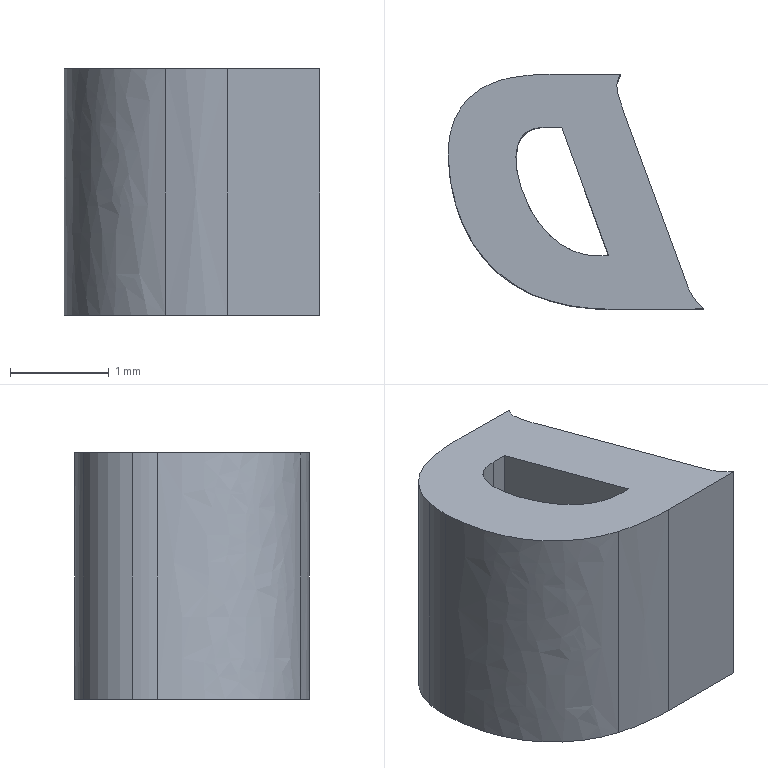Part | STEP file | lll_id1166_x_t | 1 solid | 17 faces | box 2.599 x 2.384 x 2.5 mm | volume 9.045 mm3 | plane 8 | other 6 | cylinder 3 | commonest cylinder face diameters 1.036 x1 1.35 x1 2.111 x1
STEP:
#1=CARTESIAN_POINT('',(387.606,126.033,2.35));
#2=VERTEX_POINT('',#1);
#3=CARTESIAN_POINT('',(387.495,126.033,2.35));
#4=VERTEX_POINT('',#3);
#5=CARTESIAN_POINT('',(387.495,126.033,2.35));
#6=DIRECTION('',(-1.,0.,0.));
#7=VECTOR('',#6,1.);
#8=LINE('',#5,#7);
#9=EDGE_CURVE('',#2,#4,#8,.T.);
#10=ORIENTED_EDGE('',*,*,#9,.F.);
#11=CARTESIAN_POINT('',(387.606,126.033,-0.15));
#12=VERTEX_POINT('',#11);
#13=CARTESIAN_POINT('',(387.606,126.033,-0.15));
#14=DIRECTION('',(0.,0.,-1.));
#15=VECTOR('',#14,1.);
#16=LINE('',#13,#15);
#17=EDGE_CURVE('',#2,#12,#16,.T.);
#18=ORIENTED_EDGE('',*,*,#17,.T.);
#19=CARTESIAN_POINT('',(387.495,126.033,-0.15));
#20=VERTEX_POINT('',#19);
#21=CARTESIAN_POINT('',(387.495,126.033,-0.15));
#22=DIRECTION('',(-1.,0.,0.));
#23=VECTOR('',#22,1.);
#24=LINE('',#21,#23);
#25=EDGE_CURVE('',#12,#20,#24,.T.);
#26=ORIENTED_EDGE('',*,*,#25,.T.);
#27=CARTESIAN_POINT('',(387.495,126.033,-0.15));
#28=DIRECTION('',(0.,0.,-1.));
#29=VECTOR('',#28,1.);
#30=LINE('',#27,#29);
#31=EDGE_CURVE('',#4,#20,#30,.T.);
#32=ORIENTED_EDGE('',*,*,#31,.F.);
#33=EDGE_LOOP('',(#10,#18,#26,#32));
#34=FACE_OUTER_BOUND('',#33,.T.);
#35=CARTESIAN_POINT('',(387.495,126.033,-0.15));
#36=DIRECTION('',(0.,-1.,0.));
#37=DIRECTION('',(0.,0.,-1.));
#38=AXIS2_PLACEMENT_3D('',#35,#36,#37);
#39=PLANE('',#38);
#40=ADVANCED_FACE('',(#34),#39,.F.);
#41=CARTESIAN_POINT('',(387.131,127.34,2.35));
#42=VERTEX_POINT('',#41);
#43=CARTESIAN_POINT('',(387.606,126.033,2.35));
#44=DIRECTION('',(0.3419,-0.9397,0.));
#45=VECTOR('',#44,1.);
#46=LINE('',#43,#45);
#47=EDGE_CURVE('',#42,#2,#46,.T.);
#48=ORIENTED_EDGE('',*,*,#47,.F.);
#49=CARTESIAN_POINT('',(387.131,127.34,-0.15));
#50=VERTEX_POINT('',#49);
#51=CARTESIAN_POINT('',(387.131,127.34,-0.15));
#52=DIRECTION('',(0.,0.,-1.));
#53=VECTOR('',#52,1.);
#54=LINE('',#51,#53);
#55=EDGE_CURVE('',#42,#50,#54,.T.);
#56=ORIENTED_EDGE('',*,*,#55,.T.);
#57=CARTESIAN_POINT('',(387.606,126.033,-0.15));
#58=DIRECTION('',(0.3419,-0.9397,0.));
#59=VECTOR('',#58,1.);
#60=LINE('',#57,#59);
#61=EDGE_CURVE('',#50,#12,#60,.T.);
#62=ORIENTED_EDGE('',*,*,#61,.T.);
#63=ORIENTED_EDGE('',*,*,#17,.F.);
#64=EDGE_LOOP('',(#48,#56,#62,#63));
#65=FACE_OUTER_BOUND('',#64,.T.);
#66=CARTESIAN_POINT('',(387.606,126.033,-0.15));
#67=DIRECTION('',(0.9397,0.3419,0.));
#68=DIRECTION('',(0.3419,-0.9397,0.));
#69=AXIS2_PLACEMENT_3D('',#66,#67,#68);
#70=PLANE('',#69);
#71=ADVANCED_FACE('',(#65),#70,.F.);
#72=CARTESIAN_POINT('',(386.966,127.34,2.35));
#73=VERTEX_POINT('',#72);
#74=CARTESIAN_POINT('',(387.131,127.34,2.35));
#75=DIRECTION('',(1.,0.,0.));
#76=VECTOR('',#75,1.);
#77=LINE('',#74,#76);
#78=EDGE_CURVE('',#73,#42,#77,.T.);
#79=ORIENTED_EDGE('',*,*,#78,.F.);
#80=CARTESIAN_POINT('',(386.966,127.34,-0.15));
#81=VERTEX_POINT('',#80);
#82=CARTESIAN_POINT('',(386.966,127.34,-0.15));
#83=DIRECTION('',(0.,0.,-1.));
#84=VECTOR('',#83,1.);
#85=LINE('',#82,#84);
#86=EDGE_CURVE('',#73,#81,#85,.T.);
#87=ORIENTED_EDGE('',*,*,#86,.T.);
#88=CARTESIAN_POINT('',(387.131,127.34,-0.15));
#89=DIRECTION('',(1.,0.,0.));
#90=VECTOR('',#89,1.);
#91=LINE('',#88,#90);
#92=EDGE_CURVE('',#81,#50,#91,.T.);
#93=ORIENTED_EDGE('',*,*,#92,.T.);
#94=ORIENTED_EDGE('',*,*,#55,.F.);
#95=EDGE_LOOP('',(#79,#87,#93,#94));
#96=FACE_OUTER_BOUND('',#95,.T.);
#97=CARTESIAN_POINT('',(387.131,127.34,-0.15));
#98=DIRECTION('',(0.,1.,0.));
#99=DIRECTION('',(0.,0.,1.));
#100=AXIS2_PLACEMENT_3D('',#97,#98,#99);
#101=PLANE('',#100);
#102=ADVANCED_FACE('',(#96),#101,.F.);
#103=CARTESIAN_POINT('',(386.791,127.301,2.35));
#104=VERTEX_POINT('',#103);
#105=CARTESIAN_POINT('',(386.791,127.301,2.35));
#106=CARTESIAN_POINT('',(386.817,127.316,2.35));
#107=CARTESIAN_POINT('',(386.846,127.326,2.35));
#108=CARTESIAN_POINT('',(386.905,127.337,2.35));
#109=CARTESIAN_POINT('',(386.935,127.34,2.35));
#110=CARTESIAN_POINT('',(386.966,127.34,2.35));
#111=(BOUNDED_CURVE()B_SPLINE_CURVE(3,(#105,#106,#107,#108,#109,#110),.UNSPECIFIED.,.F.,.F.)B_SPLINE_CURVE_WITH_KNOTS((4,2,4),(0.,0.4986,1.),.UNSPECIFIED.)CURVE()GEOMETRIC_REPRESENTATION_ITEM()RATIONAL_B_SPLINE_CURVE((0.5011,0.4968,0.4968,0.4996,0.4996,0.5011))REPRESENTATION_ITEM(''));
#112=EDGE_CURVE('',#104,#73,#111,.T.);
#113=ORIENTED_EDGE('',*,*,#112,.F.);
#114=CARTESIAN_POINT('',(386.791,127.301,-0.15));
#115=VERTEX_POINT('',#114);
#116=CARTESIAN_POINT('',(386.791,127.301,-0.15));
#117=DIRECTION('',(0.,0.,-1.));
#118=VECTOR('',#117,1.);
#119=LINE('',#116,#118);
#120=EDGE_CURVE('',#104,#115,#119,.T.);
#121=ORIENTED_EDGE('',*,*,#120,.T.);
#122=CARTESIAN_POINT('',(386.791,127.301,-0.15));
#123=CARTESIAN_POINT('',(386.817,127.316,-0.15));
#124=CARTESIAN_POINT('',(386.846,127.326,-0.15));
#125=CARTESIAN_POINT('',(386.905,127.337,-0.15));
#126=CARTESIAN_POINT('',(386.935,127.34,-0.15));
#127=CARTESIAN_POINT('',(386.966,127.34,-0.15));
#128=(BOUNDED_CURVE()B_SPLINE_CURVE(3,(#122,#123,#124,#125,#126,#127),.UNSPECIFIED.,.F.,.F.)B_SPLINE_CURVE_WITH_KNOTS((4,2,4),(0.,0.4986,1.),.UNSPECIFIED.)CURVE()GEOMETRIC_REPRESENTATION_ITEM()RATIONAL_B_SPLINE_CURVE((0.5011,0.4968,0.4968,0.4996,0.4996,0.5011))REPRESENTATION_ITEM(''));
#129=EDGE_CURVE('',#115,#81,#128,.T.);
#130=ORIENTED_EDGE('',*,*,#129,.T.);
#131=ORIENTED_EDGE('',*,*,#86,.F.);
#132=EDGE_LOOP('',(#113,#121,#130,#131));
#133=FACE_OUTER_BOUND('',#132,.T.);
#134=CARTESIAN_POINT('',(386.966,127.34,-0.15));
#135=CARTESIAN_POINT('',(386.935,127.34,-0.15));
#136=CARTESIAN_POINT('',(386.905,127.337,-0.15));
#137=CARTESIAN_POINT('',(386.846,127.326,-0.15));
#138=CARTESIAN_POINT('',(386.817,127.316,-0.15));
#139=CARTESIAN_POINT('',(386.791,127.301,-0.15));
#140=(BOUNDED_CURVE()B_SPLINE_CURVE(3,(#134,#135,#136,#137,#138,#139),.UNSPECIFIED.,.F.,.F.)B_SPLINE_CURVE_WITH_KNOTS((4,2,4),(0.,0.5014,1.),.UNSPECIFIED.)CURVE()GEOMETRIC_REPRESENTATION_ITEM()RATIONAL_B_SPLINE_CURVE((0.5011,0.4996,0.4996,0.4968,0.4968,0.5011))REPRESENTATION_ITEM(''));
#141=DIRECTION('',(0.,0.,1.));
#142=VECTOR('',#141,1.);
#143=SURFACE_OF_LINEAR_EXTRUSION('',#140,#142);
#144=ADVANCED_FACE('',(#133),#143,.F.);
#145=CARTESIAN_POINT('',(388.572,125.495,2.35));
#146=VERTEX_POINT('',#145);
#147=CARTESIAN_POINT('',(388.415,125.708,2.35));
#148=VERTEX_POINT('',#147);
#149=CARTESIAN_POINT('',(388.896,125.902,2.35));
#150=DIRECTION('',(0.,0.,-1.));
#151=DIRECTION('',(-1.,0.,0.));
#152=AXIS2_PLACEMENT_3D('',#149,#150,#151);
#153=CIRCLE('',#152,0.518);
#154=EDGE_CURVE('',#146,#148,#153,.T.);
#155=ORIENTED_EDGE('',*,*,#154,.F.);
#156=CARTESIAN_POINT('',(388.572,125.495,-0.15));
#157=VERTEX_POINT('',#156);
#158=CARTESIAN_POINT('',(388.578,125.492,2.35));
#159=DIRECTION('',(0.,0.,-1.));
#160=VECTOR('',#159,1.);
#161=LINE('',#158,#160);
#162=EDGE_CURVE('',#146,#157,#161,.T.);
#163=ORIENTED_EDGE('',*,*,#162,.T.);
#164=CARTESIAN_POINT('',(388.415,125.708,-0.15));
#165=VERTEX_POINT('',#164);
#166=CARTESIAN_POINT('',(388.896,125.902,-0.15));
#167=DIRECTION('',(0.,0.,-1.));
#168=DIRECTION('',(-1.,0.,0.));
#169=AXIS2_PLACEMENT_3D('',#166,#167,#168);
#170=CIRCLE('',#169,0.518);
#171=EDGE_CURVE('',#157,#165,#170,.T.);
#172=ORIENTED_EDGE('',*,*,#171,.T.);
#173=CARTESIAN_POINT('',(388.415,125.708,-0.15));
#174=DIRECTION('',(0.,0.,-1.));
#175=VECTOR('',#174,1.);
#176=LINE('',#173,#175);
#177=EDGE_CURVE('',#148,#165,#176,.T.);
#178=ORIENTED_EDGE('',*,*,#177,.F.);
#179=EDGE_LOOP('',(#155,#163,#172,#178));
#180=FACE_OUTER_BOUND('',#179,.T.);
#181=CARTESIAN_POINT('',(388.896,125.902,-0.15));
#182=DIRECTION('',(0.,0.,1.));
#183=DIRECTION('',(1.,0.,0.));
#184=AXIS2_PLACEMENT_3D('',#181,#182,#183);
#185=CYLINDRICAL_SURFACE('',#184,0.518);
#186=ADVANCED_FACE('',(#180),#185,.F.);
#187=CARTESIAN_POINT('',(387.633,125.492,2.35));
#188=VERTEX_POINT('',#187);
#189=CARTESIAN_POINT('',(388.572,125.492,2.35));
#190=DIRECTION('',(1.,0.,0.));
#191=VECTOR('',#190,1.);
#192=LINE('',#189,#191);
#193=EDGE_CURVE('',#188,#146,#192,.T.);
#194=ORIENTED_EDGE('',*,*,#193,.F.);
#195=CARTESIAN_POINT('',(387.633,125.492,-0.15));
#196=VERTEX_POINT('',#195);
#197=CARTESIAN_POINT('',(387.633,125.492,-0.15));
#198=DIRECTION('',(0.,0.,-1.));
#199=VECTOR('',#198,1.);
#200=LINE('',#197,#199);
#201=EDGE_CURVE('',#188,#196,#200,.T.);
#202=ORIENTED_EDGE('',*,*,#201,.T.);
#203=CARTESIAN_POINT('',(388.572,125.492,-0.15));
#204=DIRECTION('',(1.,0.,0.));
#205=VECTOR('',#204,1.);
#206=LINE('',#203,#205);
#207=EDGE_CURVE('',#196,#157,#206,.T.);
#208=ORIENTED_EDGE('',*,*,#207,.T.);
#209=ORIENTED_EDGE('',*,*,#162,.F.);
#210=EDGE_LOOP('',(#194,#202,#208,#209));
#211=FACE_OUTER_BOUND('',#210,.T.);
#212=CARTESIAN_POINT('',(388.572,125.492,-0.15));
#213=DIRECTION('',(0.,1.,0.));
#214=DIRECTION('',(0.,0.,1.));
#215=AXIS2_PLACEMENT_3D('',#212,#213,#214);
#216=PLANE('',#215);
#217=ADVANCED_FACE('',(#211),#216,.F.);
#218=CARTESIAN_POINT('',(387.004,125.579,2.35));
#219=VERTEX_POINT('',#218);
#220=CARTESIAN_POINT('',(387.004,125.579,2.35));
#221=CARTESIAN_POINT('',(387.105,125.548,2.35));
#222=CARTESIAN_POINT('',(387.209,125.526,2.35));
#223=CARTESIAN_POINT('',(387.42,125.499,2.35));
#224=CARTESIAN_POINT('',(387.526,125.492,2.35));
#225=CARTESIAN_POINT('',(387.633,125.492,2.35));
#226=(BOUNDED_CURVE()B_SPLINE_CURVE(3,(#220,#221,#222,#223,#224,#225),.UNSPECIFIED.,.F.,.F.)B_SPLINE_CURVE_WITH_KNOTS((4,2,4),(0.,0.4991,1.),.UNSPECIFIED.)CURVE()GEOMETRIC_REPRESENTATION_ITEM()RATIONAL_B_SPLINE_CURVE((0.5005,0.4993,0.4993,0.4998,0.4998,0.5005))REPRESENTATION_ITEM(''));
#227=EDGE_CURVE('',#219,#188,#226,.T.);
#228=ORIENTED_EDGE('',*,*,#227,.F.);
#229=CARTESIAN_POINT('',(387.004,125.579,-0.15));
#230=VERTEX_POINT('',#229);
#231=CARTESIAN_POINT('',(387.004,125.579,-0.15));
#232=DIRECTION('',(0.,0.,-1.));
#233=VECTOR('',#232,1.);
#234=LINE('',#231,#233);
#235=EDGE_CURVE('',#219,#230,#234,.T.);
#236=ORIENTED_EDGE('',*,*,#235,.T.);
#237=CARTESIAN_POINT('',(387.004,125.579,-0.15));
#238=CARTESIAN_POINT('',(387.105,125.548,-0.15));
#239=CARTESIAN_POINT('',(387.209,125.526,-0.15));
#240=CARTESIAN_POINT('',(387.42,125.499,-0.15));
#241=CARTESIAN_POINT('',(387.526,125.492,-0.15));
#242=CARTESIAN_POINT('',(387.633,125.492,-0.15));
#243=(BOUNDED_CURVE()B_SPLINE_CURVE(3,(#237,#238,#239,#240,#241,#242),.UNSPECIFIED.,.F.,.F.)B_SPLINE_CURVE_WITH_KNOTS((4,2,4),(0.,0.4991,1.),.UNSPECIFIED.)CURVE()GEOMETRIC_REPRESENTATION_ITEM()RATIONAL_B_SPLINE_CURVE((0.5005,0.4993,0.4993,0.4998,0.4998,0.5005))REPRESENTATION_ITEM(''));
#244=EDGE_CURVE('',#230,#196,#243,.T.);
#245=ORIENTED_EDGE('',*,*,#244,.T.);
#246=ORIENTED_EDGE('',*,*,#201,.F.);
#247=EDGE_LOOP('',(#228,#236,#245,#246));
#248=FACE_OUTER_BOUND('',#247,.T.);
#249=CARTESIAN_POINT('',(387.633,125.492,-0.15));
#250=CARTESIAN_POINT('',(387.526,125.492,-0.15));
#251=CARTESIAN_POINT('',(387.42,125.499,-0.15));
#252=CARTESIAN_POINT('',(387.209,125.526,-0.15));
#253=CARTESIAN_POINT('',(387.105,125.548,-0.15));
#254=CARTESIAN_POINT('',(387.004,125.579,-0.15));
#255=(BOUNDED_CURVE()B_SPLINE_CURVE(3,(#249,#250,#251,#252,#253,#254),.UNSPECIFIED.,.F.,.F.)B_SPLINE_CURVE_WITH_KNOTS((4,2,4),(0.,0.5009,1.),.UNSPECIFIED.)CURVE()GEOMETRIC_REPRESENTATION_ITEM()RATIONAL_B_SPLINE_CURVE((0.5005,0.4998,0.4998,0.4993,0.4993,0.5005))REPRESENTATION_ITEM(''));
#256=DIRECTION('',(0.,0.,1.));
#257=VECTOR('',#256,1.);
#258=SURFACE_OF_LINEAR_EXTRUSION('',#255,#257);
#259=ADVANCED_FACE('',(#248),#258,.F.);
#260=CARTESIAN_POINT('',(385.98,127.036,2.35));
#261=VERTEX_POINT('',#260);
#262=CARTESIAN_POINT('',(385.98,127.036,2.35));
#263=CARTESIAN_POINT('',(385.984,126.866,2.35));
#264=CARTESIAN_POINT('',(386.012,126.698,2.35));
#265=CARTESIAN_POINT('',(386.086,126.453,2.35));
#266=CARTESIAN_POINT('',(386.117,126.375,2.35));
#267=CARTESIAN_POINT('',(386.325,125.944,2.35));
#268=CARTESIAN_POINT('',(386.626,125.69,2.35));
#269=CARTESIAN_POINT('',(387.004,125.579,2.35));
#270=(BOUNDED_CURVE()B_SPLINE_CURVE(3,(#262,#263,#264,#265,#266,#267,#268,#269),.UNSPECIFIED.,.F.,.F.)B_SPLINE_CURVE_WITH_KNOTS((4,2,2,4),(0.,0.261,0.3919,1.),.UNSPECIFIED.)CURVE()GEOMETRIC_REPRESENTATION_ITEM()RATIONAL_B_SPLINE_CURVE((0.5005,0.4973,0.4973,0.4994,0.4994,0.4717,0.4717,0.5005))REPRESENTATION_ITEM(''));
#271=EDGE_CURVE('',#261,#219,#270,.T.);
#272=ORIENTED_EDGE('',*,*,#271,.F.);
#273=CARTESIAN_POINT('',(385.98,127.036,-0.15));
#274=VERTEX_POINT('',#273);
#275=CARTESIAN_POINT('',(385.98,127.036,-0.15));
#276=DIRECTION('',(0.,0.,-1.));
#277=VECTOR('',#276,1.);
#278=LINE('',#275,#277);
#279=EDGE_CURVE('',#261,#274,#278,.T.);
#280=ORIENTED_EDGE('',*,*,#279,.T.);
#281=CARTESIAN_POINT('',(385.98,127.036,-0.15));
#282=CARTESIAN_POINT('',(385.984,126.866,-0.15));
#283=CARTESIAN_POINT('',(386.012,126.698,-0.15));
#284=CARTESIAN_POINT('',(386.086,126.453,-0.15));
#285=CARTESIAN_POINT('',(386.117,126.375,-0.15));
#286=CARTESIAN_POINT('',(386.325,125.944,-0.15));
#287=CARTESIAN_POINT('',(386.626,125.69,-0.15));
#288=CARTESIAN_POINT('',(387.004,125.579,-0.15));
#289=(BOUNDED_CURVE()B_SPLINE_CURVE(3,(#281,#282,#283,#284,#285,#286,#287,#288),.UNSPECIFIED.,.F.,.F.)B_SPLINE_CURVE_WITH_KNOTS((4,2,2,4),(0.,0.261,0.3919,1.),.UNSPECIFIED.)CURVE()GEOMETRIC_REPRESENTATION_ITEM()RATIONAL_B_SPLINE_CURVE((0.5005,0.4973,0.4973,0.4994,0.4994,0.4717,0.4717,0.5005))REPRESENTATION_ITEM(''));
#290=EDGE_CURVE('',#274,#230,#289,.T.);
#291=ORIENTED_EDGE('',*,*,#290,.T.);
#292=ORIENTED_EDGE('',*,*,#235,.F.);
#293=EDGE_LOOP('',(#272,#280,#291,#292));
#294=FACE_OUTER_BOUND('',#293,.T.);
#295=CARTESIAN_POINT('',(387.004,125.579,-0.15));
#296=CARTESIAN_POINT('',(386.626,125.69,-0.15));
#297=CARTESIAN_POINT('',(386.325,125.944,-0.15));
#298=CARTESIAN_POINT('',(386.117,126.375,-0.15));
#299=CARTESIAN_POINT('',(386.086,126.453,-0.15));
#300=CARTESIAN_POINT('',(386.012,126.698,-0.15));
#301=CARTESIAN_POINT('',(385.984,126.866,-0.15));
#302=CARTESIAN_POINT('',(385.98,127.036,-0.15));
#303=(BOUNDED_CURVE()B_SPLINE_CURVE(3,(#295,#296,#297,#298,#299,#300,#301,#302),.UNSPECIFIED.,.F.,.F.)B_SPLINE_CURVE_WITH_KNOTS((4,2,2,4),(0.,0.6081,0.739,1.),.UNSPECIFIED.)CURVE()GEOMETRIC_REPRESENTATION_ITEM()RATIONAL_B_SPLINE_CURVE((0.5005,0.4717,0.4717,0.4994,0.4994,0.4973,0.4973,0.5005))REPRESENTATION_ITEM(''));
#304=DIRECTION('',(0.,0.,1.));
#305=VECTOR('',#304,1.);
#306=SURFACE_OF_LINEAR_EXTRUSION('',#303,#305);
#307=ADVANCED_FACE('',(#294),#306,.F.);
#308=CARTESIAN_POINT('',(386.002,127.29,2.35));
#309=VERTEX_POINT('',#308);
#310=CARTESIAN_POINT('',(387.034,127.071,2.35));
#311=DIRECTION('',(0.,0.,1.));
#312=DIRECTION('',(-1.,0.,0.));
#313=AXIS2_PLACEMENT_3D('',#310,#311,#312);
#314=CIRCLE('',#313,1.055);
#315=EDGE_CURVE('',#309,#261,#314,.T.);
#316=ORIENTED_EDGE('',*,*,#315,.F.);
#317=CARTESIAN_POINT('',(386.002,127.29,-0.15));
#318=VERTEX_POINT('',#317);
#319=CARTESIAN_POINT('',(386.002,127.29,-0.15));
#320=DIRECTION('',(0.,0.,-1.));
#321=VECTOR('',#320,1.);
#322=LINE('',#319,#321);
#323=EDGE_CURVE('',#309,#318,#322,.T.);
#324=ORIENTED_EDGE('',*,*,#323,.T.);
#325=CARTESIAN_POINT('',(387.034,127.071,-0.15));
#326=DIRECTION('',(0.,0.,1.));
#327=DIRECTION('',(-1.,0.,0.));
#328=AXIS2_PLACEMENT_3D('',#325,#326,#327);
#329=CIRCLE('',#328,1.055);
#330=EDGE_CURVE('',#318,#274,#329,.T.);
#331=ORIENTED_EDGE('',*,*,#330,.T.);
#332=ORIENTED_EDGE('',*,*,#279,.F.);
#333=EDGE_LOOP('',(#316,#324,#331,#332));
#334=FACE_OUTER_BOUND('',#333,.T.);
#335=CARTESIAN_POINT('',(387.034,127.071,-0.15));
#336=DIRECTION('',(0.,0.,1.));
#337=DIRECTION('',(1.,0.,0.));
#338=AXIS2_PLACEMENT_3D('',#335,#336,#337);
#339=CYLINDRICAL_SURFACE('',#338,1.055);
#340=ADVANCED_FACE('',(#334),#339,.T.);
#341=CARTESIAN_POINT('',(386.416,127.784,2.35));
#342=VERTEX_POINT('',#341);
#343=CARTESIAN_POINT('',(386.664,127.156,2.35));
#344=DIRECTION('',(0.,0.,1.));
#345=DIRECTION('',(-1.,0.,0.));
#346=AXIS2_PLACEMENT_3D('',#343,#344,#345);
#347=CIRCLE('',#346,0.6752);
#348=EDGE_CURVE('',#342,#309,#347,.T.);
#349=ORIENTED_EDGE('',*,*,#348,.F.);
#350=CARTESIAN_POINT('',(386.416,127.784,-0.15));
#351=VERTEX_POINT('',#350);
#352=CARTESIAN_POINT('',(386.416,127.784,-0.15));
#353=DIRECTION('',(0.,0.,-1.));
#354=VECTOR('',#353,1.);
#355=LINE('',#352,#354);
#356=EDGE_CURVE('',#342,#351,#355,.T.);
#357=ORIENTED_EDGE('',*,*,#356,.T.);
#358=CARTESIAN_POINT('',(386.664,127.156,-0.15));
#359=DIRECTION('',(0.,0.,1.));
#360=DIRECTION('',(-1.,0.,0.));
#361=AXIS2_PLACEMENT_3D('',#358,#359,#360);
#362=CIRCLE('',#361,0.6752);
#363=EDGE_CURVE('',#351,#318,#362,.T.);
#364=ORIENTED_EDGE('',*,*,#363,.T.);
#365=ORIENTED_EDGE('',*,*,#323,.F.);
#366=EDGE_LOOP('',(#349,#357,#364,#365));
#367=FACE_OUTER_BOUND('',#366,.T.);
#368=CARTESIAN_POINT('',(386.664,127.156,-0.15));
#369=DIRECTION('',(0.,0.,1.));
#370=DIRECTION('',(1.,0.,0.));
#371=AXIS2_PLACEMENT_3D('',#368,#369,#370);
#372=CYLINDRICAL_SURFACE('',#371,0.6752);
#373=ADVANCED_FACE('',(#367),#372,.T.);
#374=CARTESIAN_POINT('',(387.012,127.877,2.35));
#375=VERTEX_POINT('',#374);
#376=CARTESIAN_POINT('',(387.012,127.877,2.35));
#377=CARTESIAN_POINT('',(386.927,127.878,2.35));
#378=CARTESIAN_POINT('',(386.842,127.873,2.35));
#379=CARTESIAN_POINT('',(386.693,127.857,2.35));
#380=CARTESIAN_POINT('',(386.631,127.846,2.35));
#381=CARTESIAN_POINT('',(386.516,127.82,2.35));
#382=CARTESIAN_POINT('',(386.465,127.804,2.35));
#383=CARTESIAN_POINT('',(386.416,127.784,2.35));
#384=(BOUNDED_CURVE()B_SPLINE_CURVE(3,(#376,#377,#378,#379,#380,#381,#382,#383),.UNSPECIFIED.,.F.,.F.)B_SPLINE_CURVE_WITH_KNOTS((4,2,2,4),(0.,0.4207,0.7362,1.),.UNSPECIFIED.)CURVE()GEOMETRIC_REPRESENTATION_ITEM()RATIONAL_B_SPLINE_CURVE((0.5005,0.4999,0.4999,0.4999,0.4999,0.4994,0.4994,0.5005))REPRESENTATION_ITEM(''));
#385=EDGE_CURVE('',#375,#342,#384,.T.);
#386=ORIENTED_EDGE('',*,*,#385,.F.);
#387=CARTESIAN_POINT('',(387.012,127.877,-0.15));
#388=VERTEX_POINT('',#387);
#389=CARTESIAN_POINT('',(387.012,127.877,-0.15));
#390=DIRECTION('',(0.,0.,-1.));
#391=VECTOR('',#390,1.);
#392=LINE('',#389,#391);
#393=EDGE_CURVE('',#375,#388,#392,.T.);
#394=ORIENTED_EDGE('',*,*,#393,.T.);
#395=CARTESIAN_POINT('',(387.012,127.877,-0.15));
#396=CARTESIAN_POINT('',(386.927,127.878,-0.15));
#397=CARTESIAN_POINT('',(386.842,127.873,-0.15));
#398=CARTESIAN_POINT('',(386.693,127.857,-0.15));
#399=CARTESIAN_POINT('',(386.631,127.846,-0.15));
#400=CARTESIAN_POINT('',(386.516,127.82,-0.15));
#401=CARTESIAN_POINT('',(386.465,127.804,-0.15));
#402=CARTESIAN_POINT('',(386.416,127.784,-0.15));
#403=(BOUNDED_CURVE()B_SPLINE_CURVE(3,(#395,#396,#397,#398,#399,#400,#401,#402),.UNSPECIFIED.,.F.,.F.)B_SPLINE_CURVE_WITH_KNOTS((4,2,2,4),(0.,0.4207,0.7362,1.),.UNSPECIFIED.)CURVE()GEOMETRIC_REPRESENTATION_ITEM()RATIONAL_B_SPLINE_CURVE((0.5005,0.4999,0.4999,0.4999,0.4999,0.4994,0.4994,0.5005))REPRESENTATION_ITEM(''));
#404=EDGE_CURVE('',#388,#351,#403,.T.);
#405=ORIENTED_EDGE('',*,*,#404,.T.);
#406=ORIENTED_EDGE('',*,*,#356,.F.);
#407=EDGE_LOOP('',(#386,#394,#405,#406));
#408=FACE_OUTER_BOUND('',#407,.T.);
#409=CARTESIAN_POINT('',(386.416,127.784,-0.15));
#410=CARTESIAN_POINT('',(386.465,127.804,-0.15));
#411=CARTESIAN_POINT('',(386.516,127.82,-0.15));
#412=CARTESIAN_POINT('',(386.631,127.846,-0.15));
#413=CARTESIAN_POINT('',(386.693,127.857,-0.15));
#414=CARTESIAN_POINT('',(386.842,127.873,-0.15));
#415=CARTESIAN_POINT('',(386.927,127.878,-0.15));
#416=CARTESIAN_POINT('',(387.012,127.877,-0.15));
#417=(BOUNDED_CURVE()B_SPLINE_CURVE(3,(#409,#410,#411,#412,#413,#414,#415,#416),.UNSPECIFIED.,.F.,.F.)B_SPLINE_CURVE_WITH_KNOTS((4,2,2,4),(0.,0.2638,0.5793,1.),.UNSPECIFIED.)CURVE()GEOMETRIC_REPRESENTATION_ITEM()RATIONAL_B_SPLINE_CURVE((0.5005,0.4994,0.4994,0.4999,0.4999,0.4999,0.4999,0.5005))REPRESENTATION_ITEM(''));
#418=DIRECTION('',(0.,0.,1.));
#419=VECTOR('',#418,1.);
#420=SURFACE_OF_LINEAR_EXTRUSION('',#417,#419);
#421=ADVANCED_FACE('',(#408),#420,.F.);
#422=CARTESIAN_POINT('',(387.729,127.874,2.35));
#423=VERTEX_POINT('',#422);
#424=CARTESIAN_POINT('',(387.012,127.877,2.35));
#425=DIRECTION('',(-1.,0.,0.));
#426=VECTOR('',#425,1.);
#427=LINE('',#424,#426);
#428=EDGE_CURVE('',#423,#375,#427,.T.);
#429=ORIENTED_EDGE('',*,*,#428,.F.);
#430=CARTESIAN_POINT('',(387.729,127.874,-0.15));
#431=VERTEX_POINT('',#430);
#432=CARTESIAN_POINT('',(387.734,127.877,2.35));
#433=DIRECTION('',(0.,0.,-1.));
#434=VECTOR('',#433,1.);
#435=LINE('',#432,#434);
#436=EDGE_CURVE('',#423,#431,#435,.T.);
#437=ORIENTED_EDGE('',*,*,#436,.T.);
#438=CARTESIAN_POINT('',(387.012,127.877,-0.15));
#439=DIRECTION('',(-1.,0.,0.));
#440=VECTOR('',#439,1.);
#441=LINE('',#438,#440);
#442=EDGE_CURVE('',#431,#388,#441,.T.);
#443=ORIENTED_EDGE('',*,*,#442,.T.);
#444=ORIENTED_EDGE('',*,*,#393,.F.);
#445=EDGE_LOOP('',(#429,#437,#443,#444));
#446=FACE_OUTER_BOUND('',#445,.T.);
#447=CARTESIAN_POINT('',(387.012,127.877,-0.15));
#448=DIRECTION('',(0.,-1.,0.));
#449=DIRECTION('',(0.,0.,-1.));
#450=AXIS2_PLACEMENT_3D('',#447,#448,#449);
#451=PLANE('',#450);
#452=ADVANCED_FACE('',(#446),#451,.F.);
#453=CARTESIAN_POINT('',(387.746,127.533,2.35));
#454=VERTEX_POINT('',#453);
#455=CARTESIAN_POINT('',(387.746,127.533,2.35));
#456=CARTESIAN_POINT('',(387.741,127.547,2.35));
#457=CARTESIAN_POINT('',(387.736,127.561,2.35));
#458=CARTESIAN_POINT('',(387.723,127.6,2.35));
#459=CARTESIAN_POINT('',(387.716,127.624,2.35));
#460=CARTESIAN_POINT('',(387.706,127.66,2.35));
#461=CARTESIAN_POINT('',(387.703,127.671,2.35));
#462=CARTESIAN_POINT('',(387.698,127.692,2.35));
#463=CARTESIAN_POINT('',(387.696,127.703,2.35));
#464=CARTESIAN_POINT('',(387.692,127.723,2.35));
#465=CARTESIAN_POINT('',(387.691,127.732,2.35));
#466=CARTESIAN_POINT('',(387.69,127.755,2.35));
#467=CARTESIAN_POINT('',(387.69,127.768,2.35));
#468=CARTESIAN_POINT('',(387.694,127.814,2.35));
#469=CARTESIAN_POINT('',(387.707,127.845,2.35));
#470=CARTESIAN_POINT('',(387.729,127.871,2.35));
#471=(BOUNDED_CURVE()B_SPLINE_CURVE(3,(#455,#456,#457,#458,#459,#460,#461,#462,#463,#464,#465,#466,#467,#468,#469,#470),.UNSPECIFIED.,.F.,.F.)B_SPLINE_CURVE_WITH_KNOTS((4,2,2,2,2,2,2,4),(0.,0.1242,0.3415,0.4348,0.5281,0.6056,0.7146,1.),.UNSPECIFIED.)CURVE()GEOMETRIC_REPRESENTATION_ITEM()RATIONAL_B_SPLINE_CURVE((0.5124,0.5123,0.5123,0.5123,0.5123,0.5123,0.5123,0.5122,0.5122,0.5121,0.5121,0.5111,0.5111,0.4959,0.4959,0.5124))REPRESENTATION_ITEM(''));
#472=EDGE_CURVE('',#454,#423,#471,.T.);
#473=ORIENTED_EDGE('',*,*,#472,.F.);
#474=CARTESIAN_POINT('',(387.746,127.533,-0.15));
#475=VERTEX_POINT('',#474);
#476=CARTESIAN_POINT('',(387.746,127.533,-0.15));
#477=DIRECTION('',(0.,0.,-1.));
#478=VECTOR('',#477,1.);
#479=LINE('',#476,#478);
#480=EDGE_CURVE('',#454,#475,#479,.T.);
#481=ORIENTED_EDGE('',*,*,#480,.T.);
#482=CARTESIAN_POINT('',(387.746,127.533,-0.15));
#483=CARTESIAN_POINT('',(387.741,127.547,-0.15));
#484=CARTESIAN_POINT('',(387.736,127.561,-0.15));
#485=CARTESIAN_POINT('',(387.723,127.6,-0.15));
#486=CARTESIAN_POINT('',(387.716,127.624,-0.15));
#487=CARTESIAN_POINT('',(387.706,127.66,-0.15));
#488=CARTESIAN_POINT('',(387.703,127.671,-0.15));
#489=CARTESIAN_POINT('',(387.698,127.692,-0.15));
#490=CARTESIAN_POINT('',(387.696,127.703,-0.15));
#491=CARTESIAN_POINT('',(387.692,127.723,-0.15));
#492=CARTESIAN_POINT('',(387.691,127.732,-0.15));
#493=CARTESIAN_POINT('',(387.69,127.755,-0.15));
#494=CARTESIAN_POINT('',(387.69,127.768,-0.15));
#495=CARTESIAN_POINT('',(387.694,127.814,-0.15));
#496=CARTESIAN_POINT('',(387.707,127.845,-0.15));
#497=CARTESIAN_POINT('',(387.73,127.872,-0.15));
#498=CARTESIAN_POINT('',(387.731,127.873,-0.15));
#499=CARTESIAN_POINT('',(387.732,127.874,-0.15));
#500=(BOUNDED_CURVE()B_SPLINE_CURVE(3,(#482,#483,#484,#485,#486,#487,#488,#489,#490,#491,#492,#493,#494,#495,#496,#497,#498,#499),.UNSPECIFIED.,.F.,.F.)B_SPLINE_CURVE_WITH_KNOTS((4,2,2,2,2,2,2,2,4),(0.,0.123,0.3381,0.4305,0.5228,0.5996,0.7075,0.9901,1.),.UNSPECIFIED.)CURVE()GEOMETRIC_REPRESENTATION_ITEM()RATIONAL_B_SPLINE_CURVE((0.5124,0.5123,0.5123,0.5123,0.5123,0.5123,0.5123,0.5122,0.5122,0.5121,0.5121,0.5111,0.5111,0.4959,0.4959,0.5124,0.5124,0.5124))REPRESENTATION_ITEM(''));
#501=EDGE_CURVE('',#475,#431,#500,.T.);
#502=ORIENTED_EDGE('',*,*,#501,.T.);
#503=ORIENTED_EDGE('',*,*,#436,.F.);
#504=EDGE_LOOP('',(#473,#481,#502,#503));
#505=FACE_OUTER_BOUND('',#504,.T.);
#506=CARTESIAN_POINT('',(387.736,127.879,-0.15));
#507=CARTESIAN_POINT('',(387.735,127.878,-0.15));
#508=CARTESIAN_POINT('',(387.735,127.877,-0.15));
#509=CARTESIAN_POINT('',(387.733,127.875,-0.15));
#510=CARTESIAN_POINT('',(387.732,127.875,-0.15));
#511=CARTESIAN_POINT('',(387.731,127.873,-0.15));
#512=CARTESIAN_POINT('',(387.73,127.872,-0.15));
#513=CARTESIAN_POINT('',(387.707,127.845,-0.15));
#514=CARTESIAN_POINT('',(387.694,127.814,-0.15));
#515=CARTESIAN_POINT('',(387.69,127.768,-0.15));
#516=CARTESIAN_POINT('',(387.69,127.755,-0.15));
#517=CARTESIAN_POINT('',(387.691,127.732,-0.15));
#518=CARTESIAN_POINT('',(387.692,127.723,-0.15));
#519=CARTESIAN_POINT('',(387.696,127.703,-0.15));
#520=CARTESIAN_POINT('',(387.698,127.692,-0.15));
#521=CARTESIAN_POINT('',(387.703,127.671,-0.15));
#522=CARTESIAN_POINT('',(387.706,127.66,-0.15));
#523=CARTESIAN_POINT('',(387.716,127.624,-0.15));
#524=CARTESIAN_POINT('',(387.723,127.6,-0.15));
#525=CARTESIAN_POINT('',(387.736,127.561,-0.15));
#526=CARTESIAN_POINT('',(387.741,127.547,-0.15));
#527=CARTESIAN_POINT('',(387.746,127.533,-0.15));
#528=(BOUNDED_CURVE()B_SPLINE_CURVE(3,(#506,#507,#508,#509,#510,#511,#512,#513,#514,#515,#516,#517,#518,#519,#520,#521,#522,#523,#524,#525,#526,#527),.UNSPECIFIED.,.F.,.F.)B_SPLINE_CURVE_WITH_KNOTS((4,2,2,2,2,2,2,2,2,2,4),(0.,0.009901,0.0197,0.02941,0.3064,0.4123,0.4875,0.578,0.6686,0.8795,1.),.UNSPECIFIED.)CURVE()GEOMETRIC_REPRESENTATION_ITEM()RATIONAL_B_SPLINE_CURVE((0.5124,0.5124,0.5124,0.5124,0.5124,0.5124,0.5124,0.4959,0.4959,0.5111,0.5111,0.5121,0.5121,0.5122,0.5122,0.5123,0.5123,0.5123,0.5123,0.5123,0.5123,0.5124))REPRESENTATION_ITEM(''));
#529=DIRECTION('',(0.,0.,1.));
#530=VECTOR('',#529,1.);
#531=SURFACE_OF_LINEAR_EXTRUSION('',#528,#530);
#532=ADVANCED_FACE('',(#505),#531,.F.);
#533=CARTESIAN_POINT('',(387.746,127.533,2.35));
#534=DIRECTION('',(-0.3441,0.9389,0.));
#535=VECTOR('',#534,1.);
#536=LINE('',#533,#535);
#537=EDGE_CURVE('',#148,#454,#536,.T.);
#538=ORIENTED_EDGE('',*,*,#537,.F.);
#539=ORIENTED_EDGE('',*,*,#177,.T.);
#540=CARTESIAN_POINT('',(387.746,127.533,-0.15));
#541=DIRECTION('',(-0.3441,0.9389,0.));
#542=VECTOR('',#541,1.);
#543=LINE('',#540,#542);
#544=EDGE_CURVE('',#165,#475,#543,.T.);
#545=ORIENTED_EDGE('',*,*,#544,.T.);
#546=ORIENTED_EDGE('',*,*,#480,.F.);
#547=EDGE_LOOP('',(#538,#539,#545,#546));
#548=FACE_OUTER_BOUND('',#547,.T.);
#549=CARTESIAN_POINT('',(387.746,127.533,-0.15));
#550=DIRECTION('',(-0.9389,-0.3441,0.));
#551=DIRECTION('',(-0.3441,0.9389,0.));
#552=AXIS2_PLACEMENT_3D('',#549,#550,#551);
#553=PLANE('',#552);
#554=ADVANCED_FACE('',(#548),#553,.F.);
#555=CARTESIAN_POINT('',(387.495,126.033,2.35));
#556=CARTESIAN_POINT('',(387.414,126.033,2.35));
#557=CARTESIAN_POINT('',(387.335,126.047,2.35));
#558=CARTESIAN_POINT('',(387.176,126.11,2.35));
#559=CARTESIAN_POINT('',(387.099,126.158,2.35));
#560=CARTESIAN_POINT('',(386.966,126.279,2.35));
#561=CARTESIAN_POINT('',(386.908,126.348,2.35));
#562=CARTESIAN_POINT('',(386.785,126.542,2.35));
#563=CARTESIAN_POINT('',(386.731,126.67,2.35));
#564=CARTESIAN_POINT('',(386.683,126.854,2.35));
#565=CARTESIAN_POINT('',(386.674,126.903,2.35));
#566=CARTESIAN_POINT('',(386.666,126.982,2.35));
#567=CARTESIAN_POINT('',(386.665,127.012,2.35));
#568=CARTESIAN_POINT('',(386.667,127.077,2.35));
#569=CARTESIAN_POINT('',(386.672,127.112,2.35));
#570=CARTESIAN_POINT('',(386.687,127.17,2.35));
#571=CARTESIAN_POINT('',(386.696,127.194,2.35));
#572=CARTESIAN_POINT('',(386.727,127.252,2.35));
#573=CARTESIAN_POINT('',(386.756,127.281,2.35));
#574=CARTESIAN_POINT('',(386.791,127.301,2.35));
#575=(BOUNDED_CURVE()B_SPLINE_CURVE(3,(#555,#556,#557,#558,#559,#560,#561,#562,#563,#564,#565,#566,#567,#568,#569,#570,#571,#572,#573,#574),.UNSPECIFIED.,.F.,.F.)B_SPLINE_CURVE_WITH_KNOTS((4,2,2,2,2,2,2,2,2,4),(0.,0.1351,0.2884,0.4424,0.6837,0.7706,0.8228,0.8841,0.9283,1.),.UNSPECIFIED.)CURVE()GEOMETRIC_REPRESENTATION_ITEM()RATIONAL_B_SPLINE_CURVE((0.5011,0.4952,0.4952,0.4957,0.4957,0.4981,0.4981,0.497,0.497,0.5001,0.5001,0.5004,0.5004,0.499,0.499,0.4987,0.4987,0.4882,0.4882,0.5011))REPRESENTATION_ITEM(''));
#576=EDGE_CURVE('',#4,#104,#575,.T.);
#577=ORIENTED_EDGE('',*,*,#576,.F.);
#578=ORIENTED_EDGE('',*,*,#31,.T.);
#579=CARTESIAN_POINT('',(387.495,126.033,-0.15));
#580=CARTESIAN_POINT('',(387.414,126.033,-0.15));
#581=CARTESIAN_POINT('',(387.335,126.047,-0.15));
#582=CARTESIAN_POINT('',(387.176,126.11,-0.15));
#583=CARTESIAN_POINT('',(387.099,126.158,-0.15));
#584=CARTESIAN_POINT('',(386.966,126.279,-0.15));
#585=CARTESIAN_POINT('',(386.908,126.348,-0.15));
#586=CARTESIAN_POINT('',(386.785,126.542,-0.15));
#587=CARTESIAN_POINT('',(386.731,126.67,-0.15));
#588=CARTESIAN_POINT('',(386.683,126.854,-0.15));
#589=CARTESIAN_POINT('',(386.674,126.903,-0.15));
#590=CARTESIAN_POINT('',(386.666,126.982,-0.15));
#591=CARTESIAN_POINT('',(386.665,127.012,-0.15));
#592=CARTESIAN_POINT('',(386.667,127.077,-0.15));
#593=CARTESIAN_POINT('',(386.672,127.112,-0.15));
#594=CARTESIAN_POINT('',(386.687,127.17,-0.15));
#595=CARTESIAN_POINT('',(386.696,127.194,-0.15));
#596=CARTESIAN_POINT('',(386.727,127.252,-0.15));
#597=CARTESIAN_POINT('',(386.756,127.281,-0.15));
#598=CARTESIAN_POINT('',(386.791,127.301,-0.15));
#599=(BOUNDED_CURVE()B_SPLINE_CURVE(3,(#579,#580,#581,#582,#583,#584,#585,#586,#587,#588,#589,#590,#591,#592,#593,#594,#595,#596,#597,#598),.UNSPECIFIED.,.F.,.F.)B_SPLINE_CURVE_WITH_KNOTS((4,2,2,2,2,2,2,2,2,4),(0.,0.1351,0.2884,0.4424,0.6837,0.7706,0.8228,0.8841,0.9283,1.),.UNSPECIFIED.)CURVE()GEOMETRIC_REPRESENTATION_ITEM()RATIONAL_B_SPLINE_CURVE((0.5011,0.4952,0.4952,0.4957,0.4957,0.4981,0.4981,0.497,0.497,0.5001,0.5001,0.5004,0.5004,0.499,0.499,0.4987,0.4987,0.4882,0.4882,0.5011))REPRESENTATION_ITEM(''));
#600=EDGE_CURVE('',#20,#115,#599,.T.);
#601=ORIENTED_EDGE('',*,*,#600,.T.);
#602=ORIENTED_EDGE('',*,*,#120,.F.);
#603=EDGE_LOOP('',(#577,#578,#601,#602));
#604=FACE_OUTER_BOUND('',#603,.T.);
#605=CARTESIAN_POINT('',(386.791,127.301,-0.15));
#606=CARTESIAN_POINT('',(386.756,127.281,-0.15));
#607=CARTESIAN_POINT('',(386.727,127.252,-0.15));
#608=CARTESIAN_POINT('',(386.696,127.194,-0.15));
#609=CARTESIAN_POINT('',(386.687,127.17,-0.15));
#610=CARTESIAN_POINT('',(386.672,127.112,-0.15));
#611=CARTESIAN_POINT('',(386.667,127.077,-0.15));
#612=CARTESIAN_POINT('',(386.665,127.012,-0.15));
#613=CARTESIAN_POINT('',(386.666,126.982,-0.15));
#614=CARTESIAN_POINT('',(386.674,126.903,-0.15));
#615=CARTESIAN_POINT('',(386.683,126.854,-0.15));
#616=CARTESIAN_POINT('',(386.731,126.67,-0.15));
#617=CARTESIAN_POINT('',(386.785,126.542,-0.15));
#618=CARTESIAN_POINT('',(386.908,126.348,-0.15));
#619=CARTESIAN_POINT('',(386.966,126.279,-0.15));
#620=CARTESIAN_POINT('',(387.099,126.158,-0.15));
#621=CARTESIAN_POINT('',(387.176,126.11,-0.15));
#622=CARTESIAN_POINT('',(387.335,126.047,-0.15));
#623=CARTESIAN_POINT('',(387.414,126.033,-0.15));
#624=CARTESIAN_POINT('',(387.495,126.033,-0.15));
#625=(BOUNDED_CURVE()B_SPLINE_CURVE(3,(#605,#606,#607,#608,#609,#610,#611,#612,#613,#614,#615,#616,#617,#618,#619,#620,#621,#622,#623,#624),.UNSPECIFIED.,.F.,.F.)B_SPLINE_CURVE_WITH_KNOTS((4,2,2,2,2,2,2,2,2,4),(0.,0.07173,0.1159,0.1772,0.2294,0.3163,0.5576,0.7116,0.8649,1.),.UNSPECIFIED.)CURVE()GEOMETRIC_REPRESENTATION_ITEM()RATIONAL_B_SPLINE_CURVE((0.5011,0.4882,0.4882,0.4987,0.4987,0.499,0.499,0.5004,0.5004,0.5001,0.5001,0.497,0.497,0.4981,0.4981,0.4957,0.4957,0.4952,0.4952,0.5011))REPRESENTATION_ITEM(''));
#626=DIRECTION('',(0.,0.,1.));
#627=VECTOR('',#626,1.);
#628=SURFACE_OF_LINEAR_EXTRUSION('',#625,#627);
#629=ADVANCED_FACE('',(#604),#628,.F.);
#630=ORIENTED_EDGE('',*,*,#171,.F.);
#631=ORIENTED_EDGE('',*,*,#207,.F.);
#632=ORIENTED_EDGE('',*,*,#244,.F.);
#633=ORIENTED_EDGE('',*,*,#290,.F.);
#634=ORIENTED_EDGE('',*,*,#330,.F.);
#635=ORIENTED_EDGE('',*,*,#363,.F.);
#636=ORIENTED_EDGE('',*,*,#404,.F.);
#637=ORIENTED_EDGE('',*,*,#442,.F.);
#638=ORIENTED_EDGE('',*,*,#501,.F.);
#639=ORIENTED_EDGE('',*,*,#544,.F.);
#640=EDGE_LOOP('',(#630,#631,#632,#633,#634,#635,#636,#637,#638,#639));
#641=FACE_BOUND('',#640,.T.);
#642=ORIENTED_EDGE('',*,*,#25,.F.);
#643=ORIENTED_EDGE('',*,*,#61,.F.);
#644=ORIENTED_EDGE('',*,*,#92,.F.);
#645=ORIENTED_EDGE('',*,*,#129,.F.);
#646=ORIENTED_EDGE('',*,*,#600,.F.);
#647=EDGE_LOOP('',(#642,#643,#644,#645,#646));
#648=FACE_BOUND('',#647,.T.);
#649=CARTESIAN_POINT('',(388.896,125.902,-0.15));
#650=DIRECTION('',(0.,0.,1.));
#651=DIRECTION('',(1.,0.,0.));
#652=AXIS2_PLACEMENT_3D('',#649,#650,#651);
#653=PLANE('',#652);
#654=ADVANCED_FACE('',(#641,#648),#653,.F.);
#655=ORIENTED_EDGE('',*,*,#154,.T.);
#656=ORIENTED_EDGE('',*,*,#537,.T.);
#657=ORIENTED_EDGE('',*,*,#472,.T.);
#658=ORIENTED_EDGE('',*,*,#428,.T.);
#659=ORIENTED_EDGE('',*,*,#385,.T.);
#660=ORIENTED_EDGE('',*,*,#348,.T.);
#661=ORIENTED_EDGE('',*,*,#315,.T.);
#662=ORIENTED_EDGE('',*,*,#271,.T.);
#663=ORIENTED_EDGE('',*,*,#227,.T.);
#664=ORIENTED_EDGE('',*,*,#193,.T.);
#665=EDGE_LOOP('',(#655,#656,#657,#658,#659,#660,#661,#662,#663,#664));
#666=FACE_BOUND('',#665,.T.);
#667=ORIENTED_EDGE('',*,*,#9,.T.);
#668=ORIENTED_EDGE('',*,*,#576,.T.);
#669=ORIENTED_EDGE('',*,*,#112,.T.);
#670=ORIENTED_EDGE('',*,*,#78,.T.);
#671=ORIENTED_EDGE('',*,*,#47,.T.);
#672=EDGE_LOOP('',(#667,#668,#669,#670,#671));
#673=FACE_BOUND('',#672,.T.);
#674=CARTESIAN_POINT('',(388.896,125.902,2.35));
#675=DIRECTION('',(0.,0.,1.));
#676=DIRECTION('',(1.,0.,0.));
#677=AXIS2_PLACEMENT_3D('',#674,#675,#676);
#678=PLANE('',#677);
#679=ADVANCED_FACE('',(#666,#673),#678,.T.);
#680=CLOSED_SHELL('',(#40,#71,#102,#144,#186,#217,#259,#307,#340,#373,#421,#452,#532,#554,#629,#654,#679));
#681=MANIFOLD_SOLID_BREP('',#680);
#682=(LENGTH_UNIT()NAMED_UNIT(*)SI_UNIT(.MILLI.,.METRE.));
#683=UNCERTAINTY_MEASURE_WITH_UNIT(LENGTH_MEASURE(0.01393),#682,'','');
#684=(NAMED_UNIT(*)PLANE_ANGLE_UNIT()SI_UNIT($,.RADIAN.));
#685=PLANE_ANGLE_MEASURE_WITH_UNIT(PLANE_ANGLE_MEASURE(0.01745),#684);
#686=DIMENSIONAL_EXPONENTS(0.,0.,0.,0.,0.,0.,0.);
#687=(CONVERSION_BASED_UNIT('DEGREE',#685)NAMED_UNIT(#686)PLANE_ANGLE_UNIT());
#688=(NAMED_UNIT(*)SI_UNIT($,.STERADIAN.)SOLID_ANGLE_UNIT());
#689=(GEOMETRIC_REPRESENTATION_CONTEXT(3)GLOBAL_UNCERTAINTY_ASSIGNED_CONTEXT((#683))GLOBAL_UNIT_ASSIGNED_CONTEXT((#682,#687,#688))REPRESENTATION_CONTEXT('',''));
#690=ADVANCED_BREP_SHAPE_REPRESENTATION('',(#681),#689);